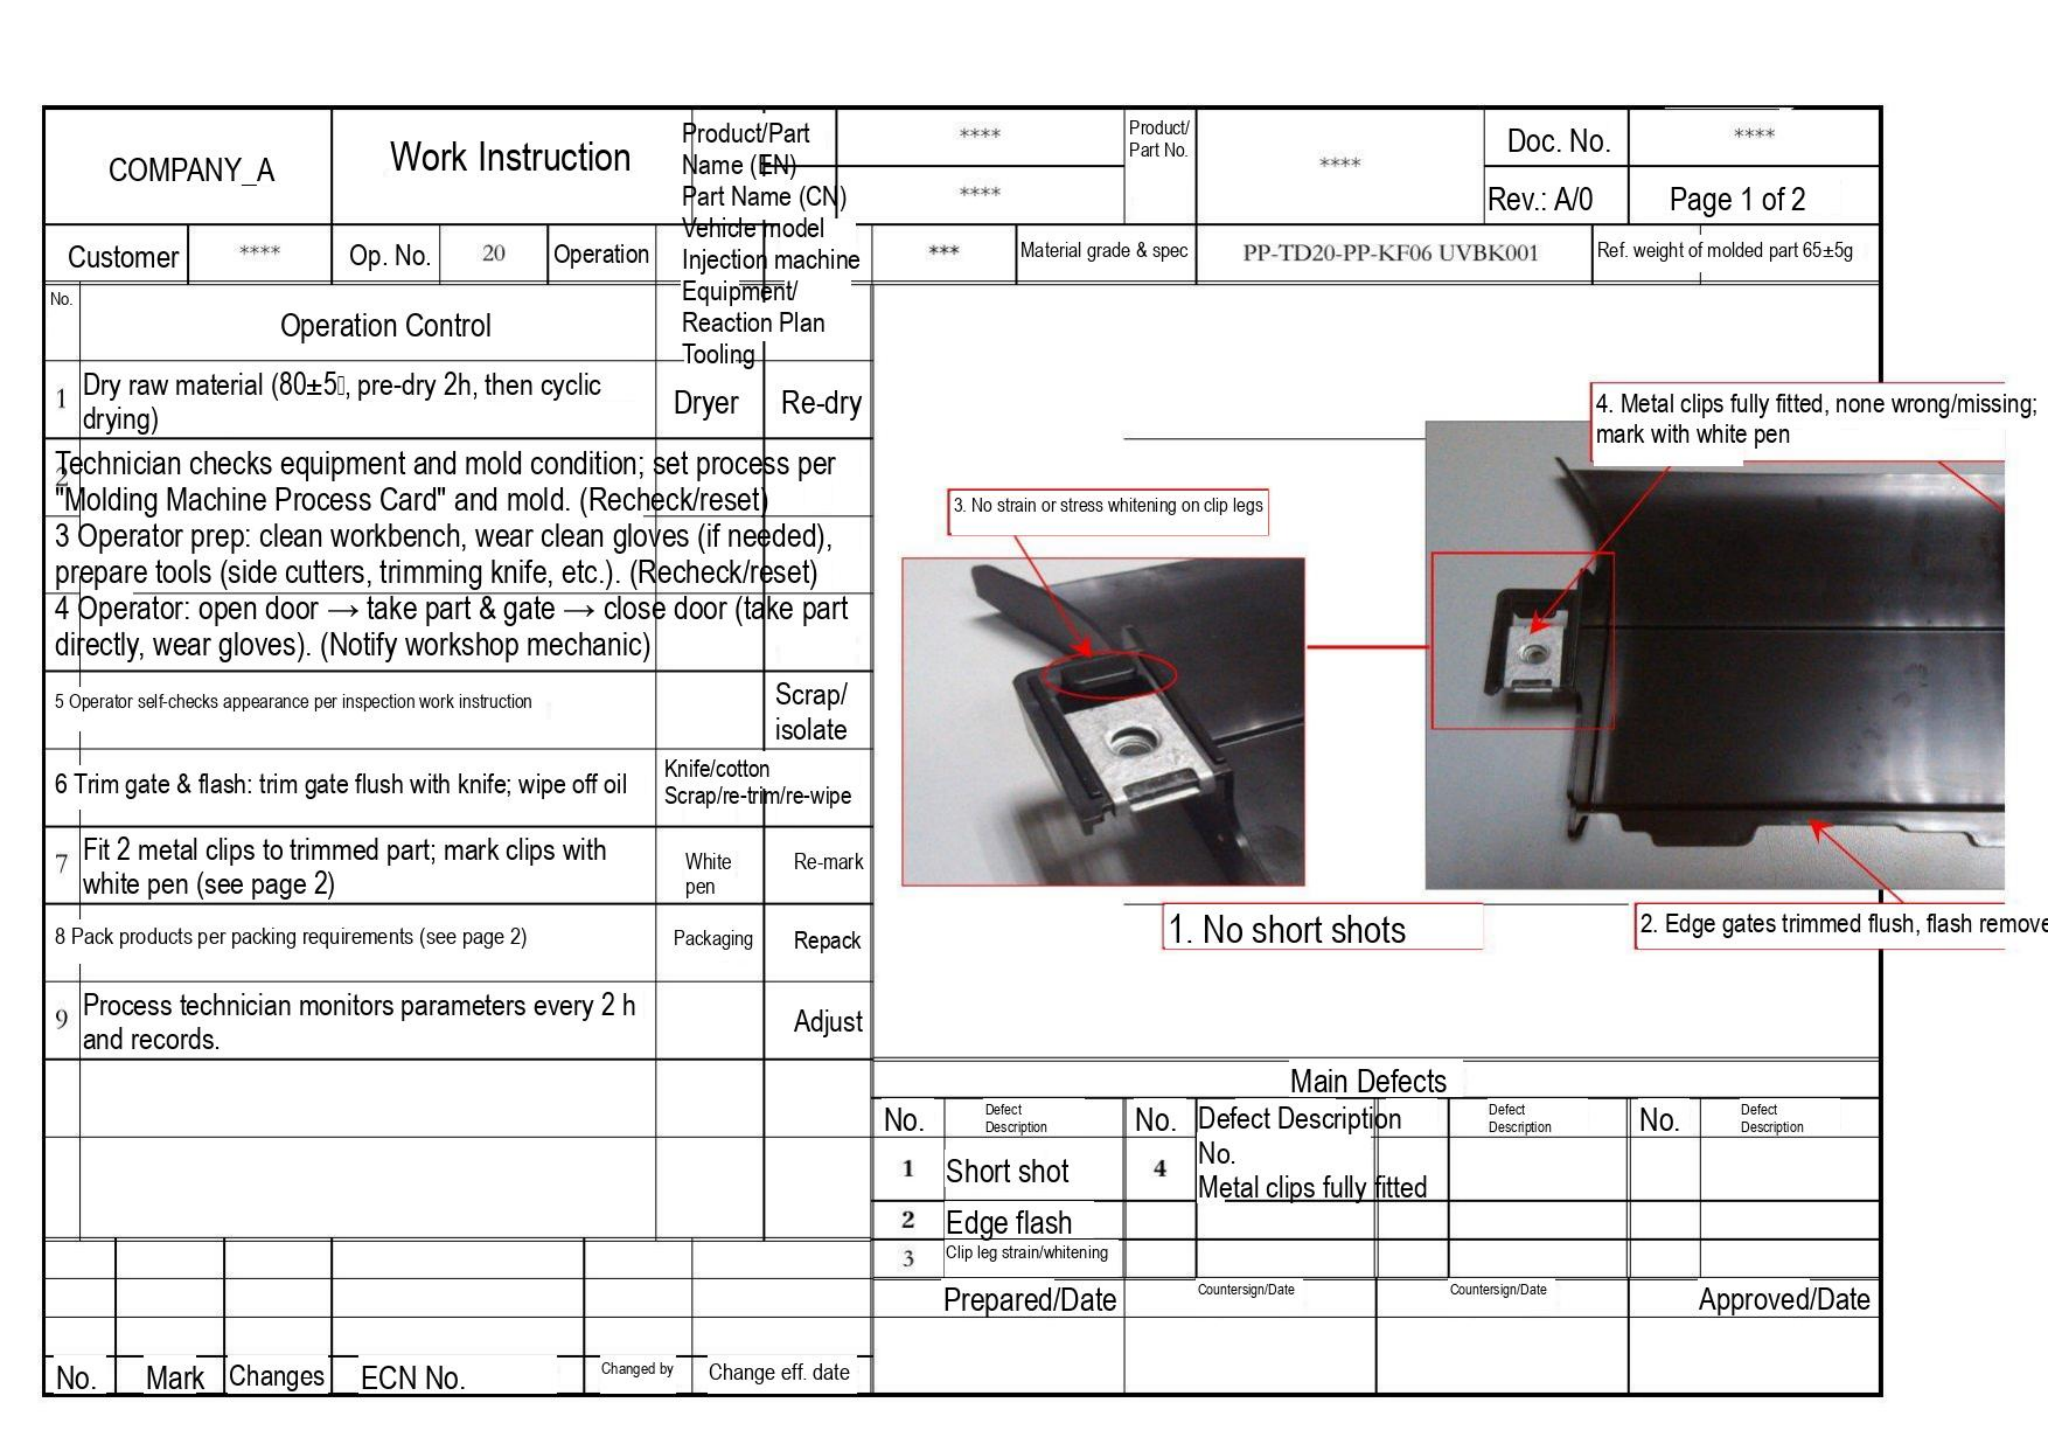| COMPANY_A | Work Instruction | Product/Part Name (EN) | **** | Product/ Part No. | **** | Doc. No. | **** |
|---|---|---|---|---|---|---|---|
| | | Part Name (CN) | **** | | | Rev.: A/0 | Page 1 of 2 |

| Customer | **** | Op. No. | 20 | Operation | Vehicle model Injection machine | *** | Material grade & spec | PP-TD20-PP-KF06 UVBK001 | Ref. weight of molded part 65±5g |
|---|---|---|---|---|---|---|---|---|---|

| No. | Operation Control | Equipment/ Tooling | Reaction Plan |
|---|---|---|---|
| 1 | Dry raw material (80±5, pre-dry 2h, then cyclic drying) | Dryer | Re-dry |
| 2 | Technician checks equipment and mold condition; set process per "Molding Machine Process Card" and mold. (Recheck/reset) | | |
| 3 | Operator prep: clean workbench, wear clean gloves (if needed), prepare tools (side cutters, trimming knife, etc.). (Recheck/reset) | | |
| 4 | Operator: open door → take part & gate → close door (take part directly, wear gloves). (Notify workshop mechanic) | | |
| 5 | Operator self-checks appearance per inspection work instruction | | Scrap/ isolate |
| 6 | Trim gate & flash: trim gate flush with knife; wipe off oil | Knife/cotton | Scrap/re-trim/re-wipe |
| 7 | Fit 2 metal clips to trimmed part; mark clips with white pen (see page 2) | White pen | Re-mark |
| 8 | Pack products per packing requirements (see page 2) | Packaging | Repack |
| 9 | Process technician monitors parameters every 2 h and records. | | Adjust |
| | | | |
| | | | |

3. No strain or stress whitening on clip legs

4. Metal clips fully fitted, none wrong/missing; mark with white pen

1. No short shots

2. Edge gates trimmed flush, flash remove

Main Defects

| No. | Defect Description | No. | Defect Description | Defect Description | No. | Defect Description |
|---|---|---|---|---|---|---|
| 1 | Short shot | 4 | No. Metal clips fully fitted | | | |
| 2 | Edge flash | | | | | |
| 3 | Clip leg strain/whitening | | | | | |

| No. | Mark | Changes | ECN No. | Changed by | Change eff. date |
|---|---|---|---|---|---|
| | | | | | |

| Prepared/Date | Countersign/Date | Countersign/Date | Approved/Date |
|---|---|---|---|
| | | | |
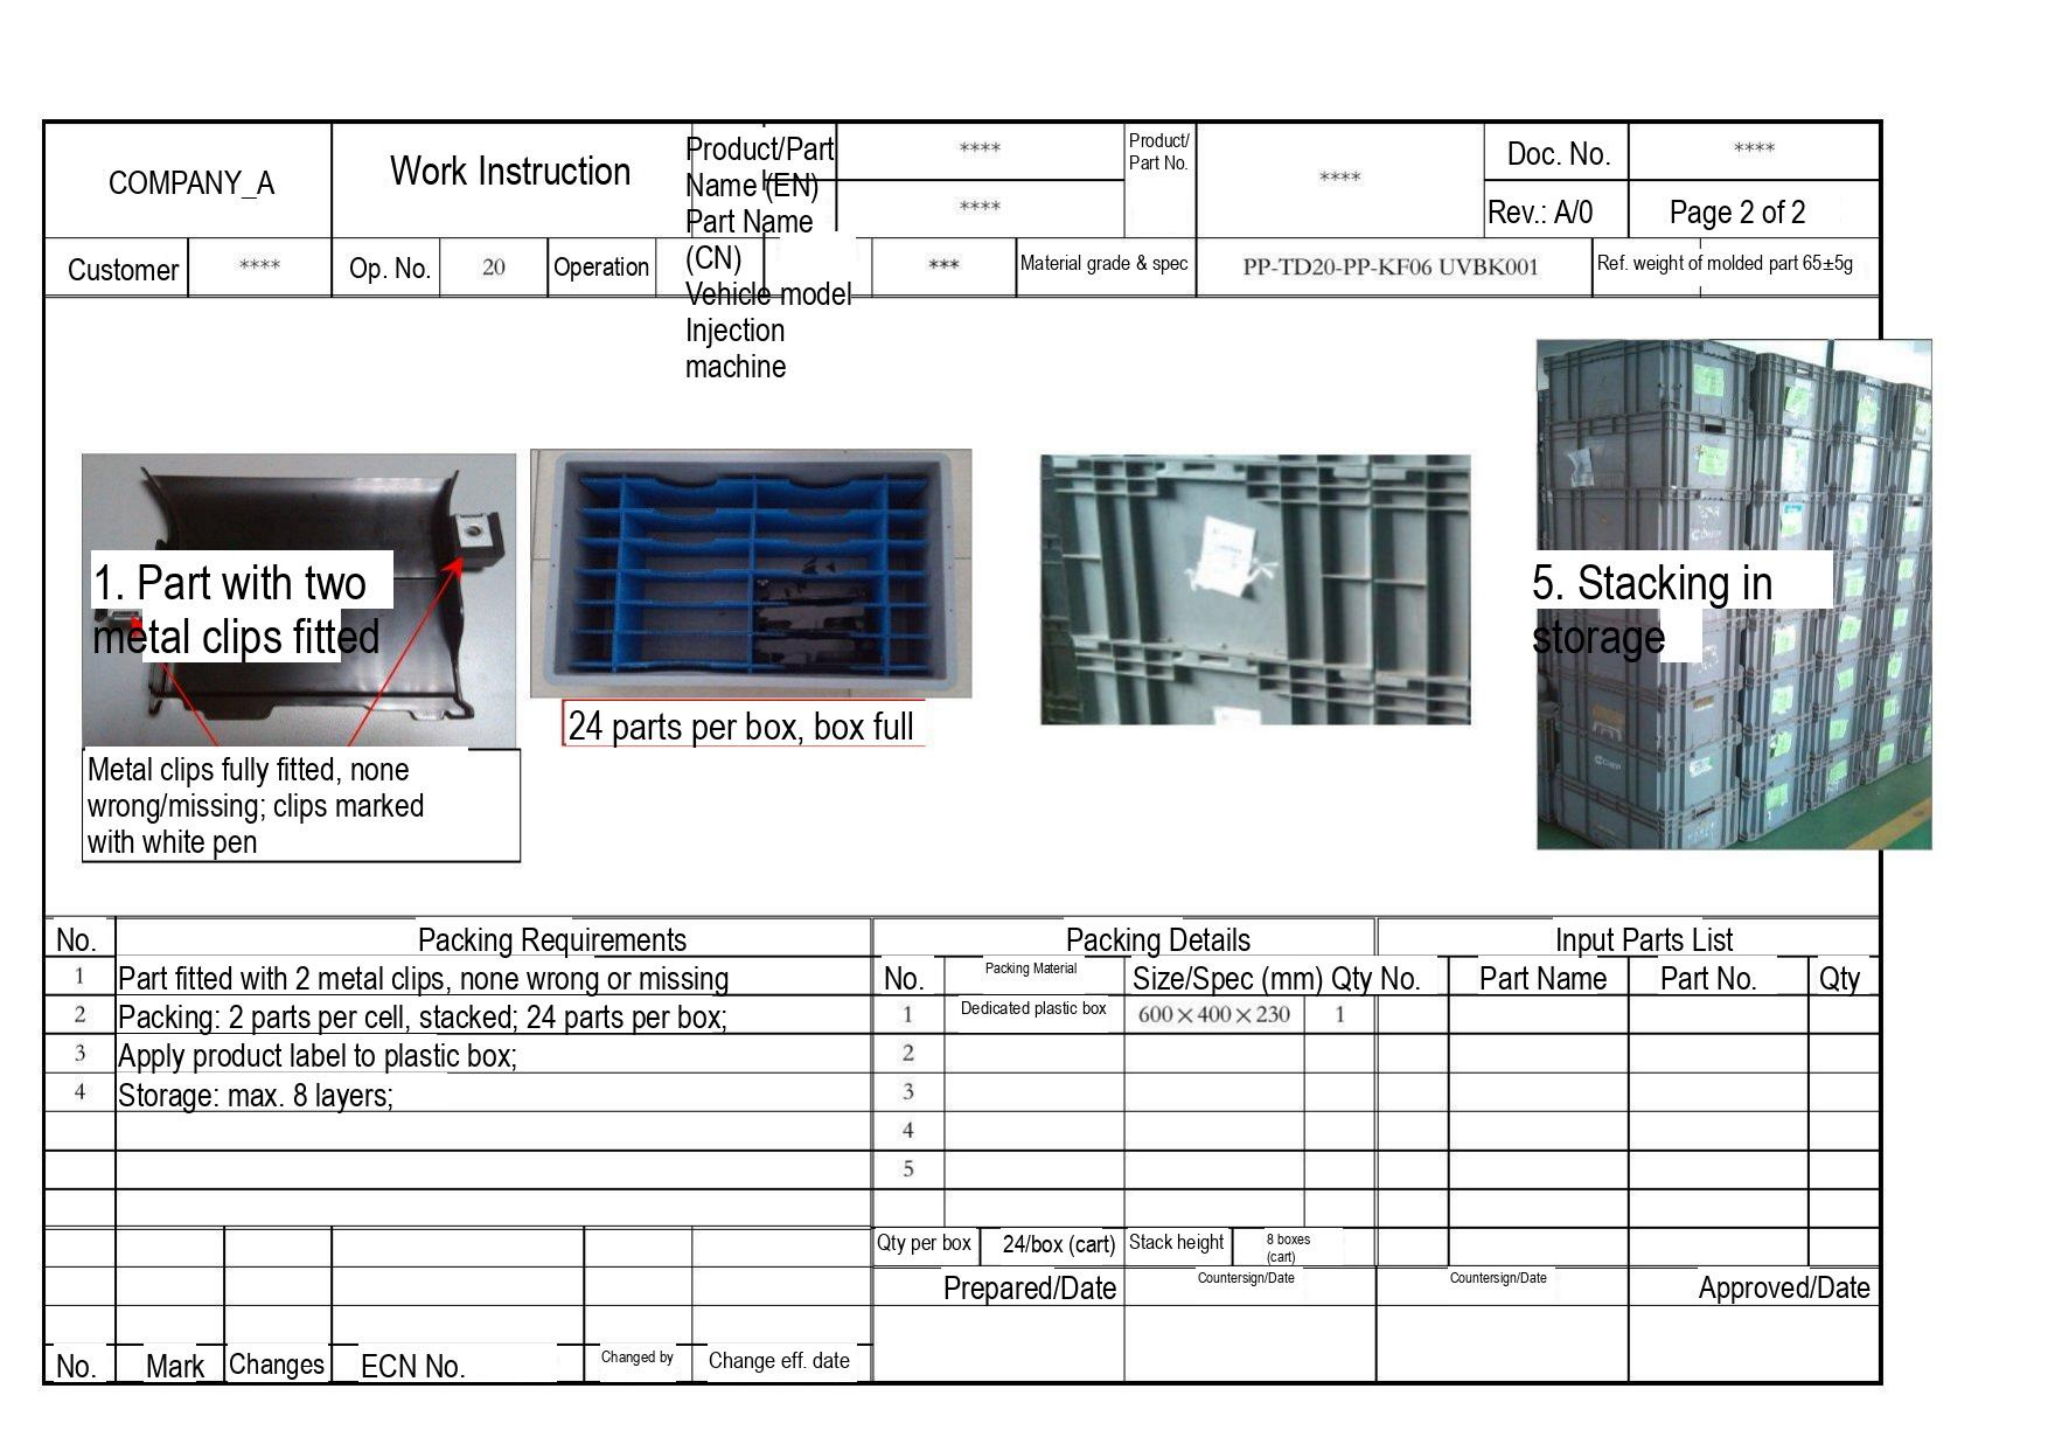COMPANY_A

Work Instruction

| Product/Part Name (EN) | **** | Product/ Part No. | **** | Doc. No. | **** |
|---|---|---|---|---|---|
| Part Name (CN) | **** | | | Rev.: A/0 | Page 2 of 2 |

| Customer | **** | Op. No. | 20 | Operation | | Vehicle model | *** | Material grade & spec | PP-TD20-PP-KF06 UVBK001 | Ref. weight of molded part 65±5g |
|---|---|---|---|---|---|---|---|---|---|---|

Injection machine

1. Part with two metal clips fitted

Metal clips fully fitted, none wrong/missing; clips marked with white pen

24 parts per box, box full

5. Stacking in storage

| No. | Packing Requirements |
|---|---|
| 1 | Part fitted with 2 metal clips, none wrong or missing |
| 2 | Packing: 2 parts per cell, stacked; 24 parts per box; |
| 3 | Apply product label to plastic box; |
| 4 | Storage: max. 8 layers; |
| | |
| | |
| | |

Packing Details

| No. | Packing Material | Size/Spec (mm) | Qty |
|---|---|---|---|
| 1 | Dedicated plastic box | 600×400×230 | 1 |
| 2 | | | |
| 3 | | | |
| 4 | | | |
| 5 | | | |
| | | | |
| Qty per box | 24/box (cart) | Stack height | 8 boxes (cart) |

Input Parts List

| No. | Part Name | Part No. | Qty |
|---|---|---|---|
| | | | |
| | | | |
| | | | |
| | | | |
| | | | |
| | | | |
| | | | |

| No. | Mark | Changes | ECN No. | Changed by | Change eff. date |
|---|---|---|---|---|---|
| | | | | | |
| | | | | | |

| Prepared/Date | Countersign/Date | Countersign/Date | Approved/Date |
|---|---|---|---|
| | | | |
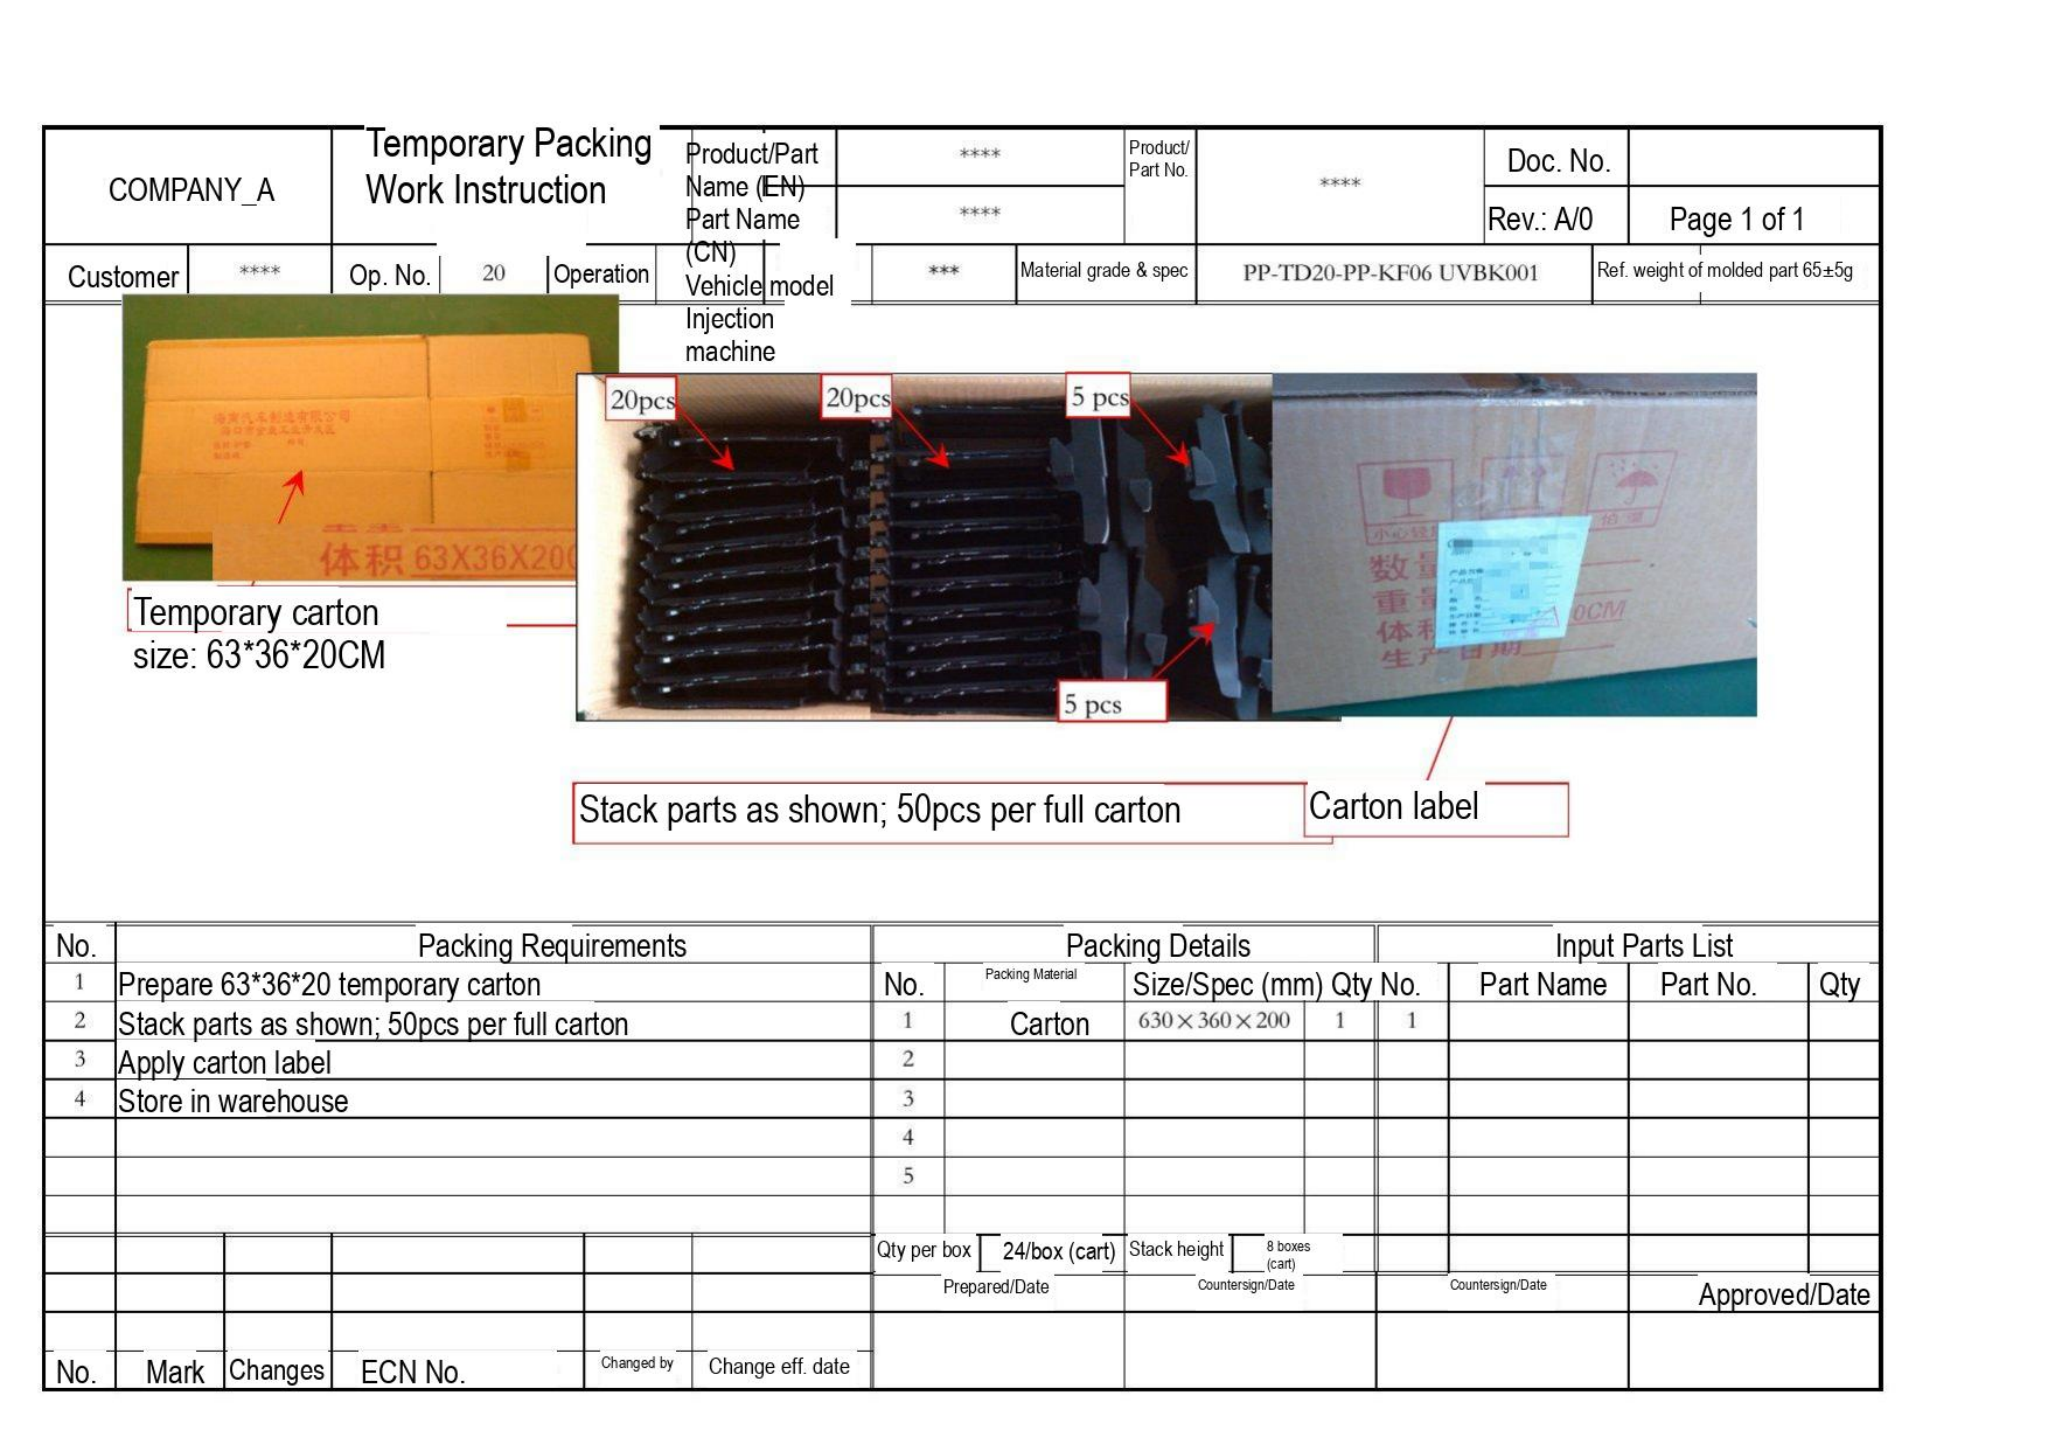| COMPANY_A | Temporary Packing Work Instruction | Product/Part Name (EN) | **** | Product/ Part No. | **** | Doc. No. | |
|---|---|---|---|---|---|---|---|
| | | Part Name (CN) | **** | | | Rev.: A/0 | Page 1 of 1 |

| Customer | **** | Op. No. | 20 | Operation | Injection machine | Vehicle model | *** | Material grade & spec | PP-TD20-PP-KF06 UVBK001 | Ref. weight of molded part 65±5g |
|---|---|---|---|---|---|---|---|---|---|---|

体积 63X36X20

Temporary carton size: 63*36*20CM

20pcs

20pcs

5 pcs

5 pcs

数量

重量

体积

0CM

Stack parts as shown; 50pcs per full carton

Carton label

| No. | Packing Requirements | No. | Packing Material | Size/Spec (mm) | Qty | No. | Part Name | Part No. | Qty |
|---|---|---|---|---|---|---|---|---|---|
| 1 | Prepare 63*36*20 temporary carton | 1 | Carton | 630×360×200 | 1 | 1 | | | |
| 2 | Stack parts as shown; 50pcs per full carton | 2 | | | | | | | |
| 3 | Apply carton label | 3 | | | | | | | |
| 4 | Store in warehouse | 4 | | | | | | | |
| | | 5 | | | | | | | |

Qty per box 24/box (cart) Stack height 8 boxes (cart)

| Prepared/Date | Countersign/Date | Countersign/Date | Approved/Date |
|---|---|---|---|
| | | | |

| No. | Mark | Changes | ECN No. | Changed by | Change eff. date |
|---|---|---|---|---|---|
| | | | | | |
| | | | | | |
| | | | | | |
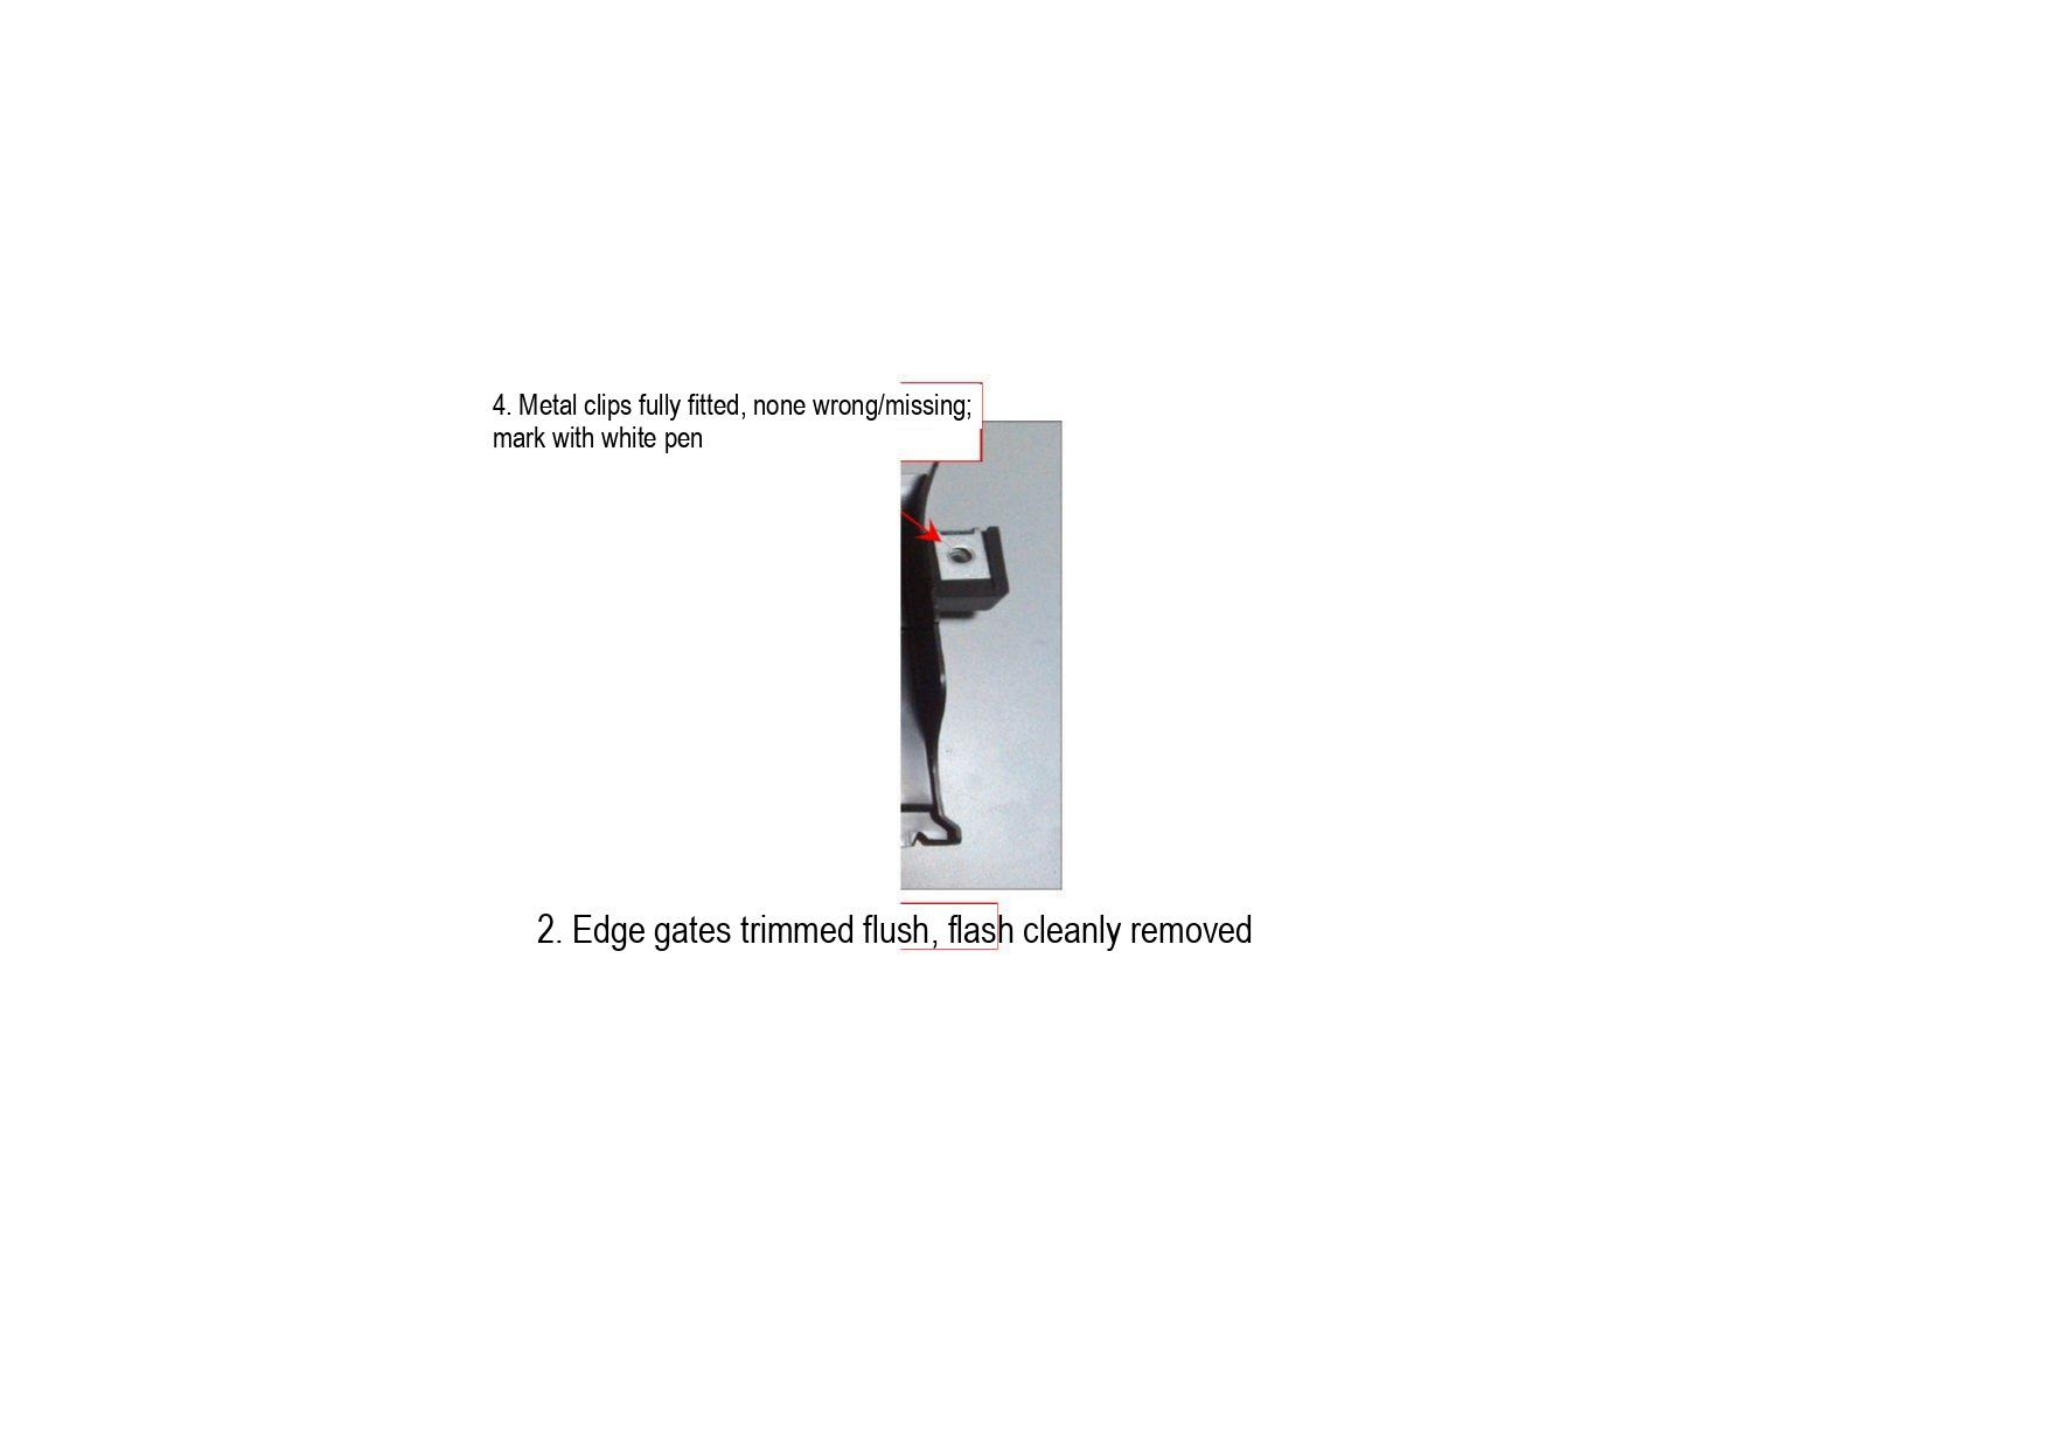4. Metal clips fully fitted, none wrong/missing; mark with white pen

2. Edge gates trimmed flush, flash cleanly removed